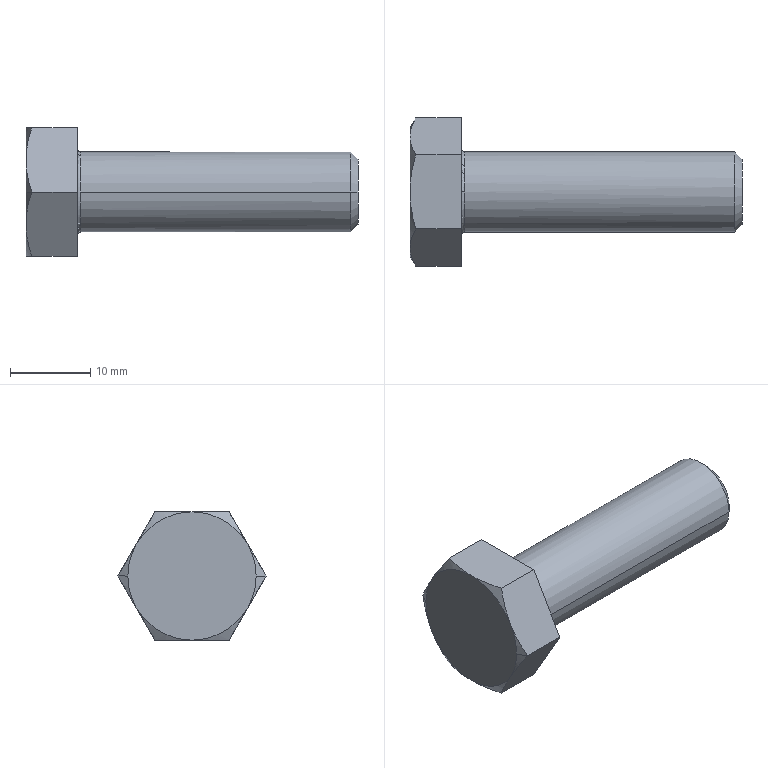Part | STEP file | KS B 1002 - C  M 10 x 35 | 1 solid | 23 faces | box 41.4 x 18.475 x 16 mm | volume 4152 mm3 | cone 10 | plane 9 | torus 2 | cylinder 2 | commonest cylinder face diameters 10 x2